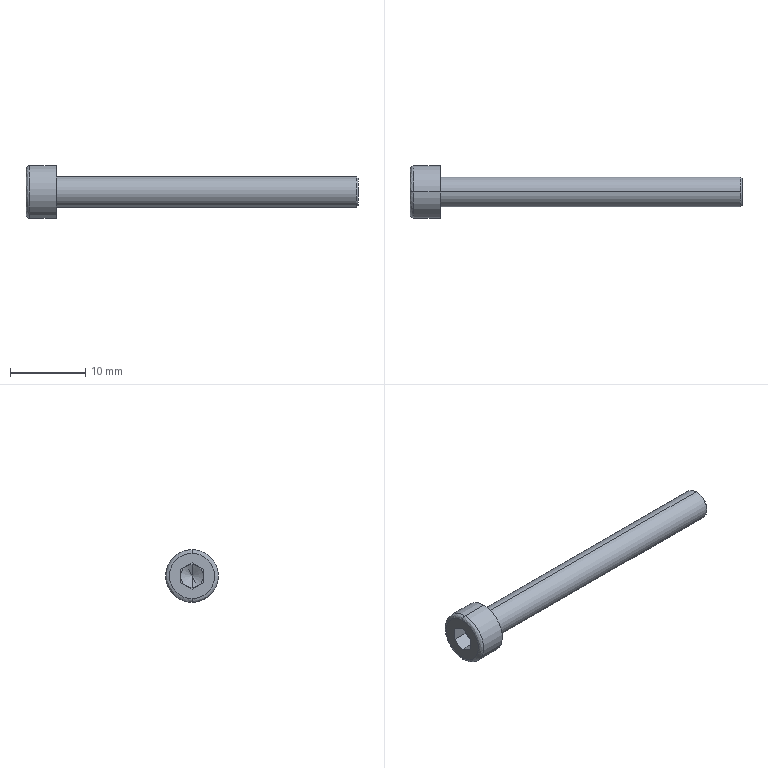Part | STEP file | hexagon socket head cap screws gb_GB_FASTENER_SCREWS_HSHCS M4X40-N | 1 solid | 25 faces | box 44 x 7 x 7 mm | volume 637.59 mm3 | plane 15 | cylinder 4 | cone 4 | spline 2 | commonest cylinder face diameters 4 x2 7 x2
STEP:
#1=CARTESIAN_POINT('',(0.5,0.,3.5));
#2=VERTEX_POINT('',#1);
#3=CARTESIAN_POINT('',(0.5,0.,-3.5));
#4=VERTEX_POINT('',#3);
#5=CARTESIAN_POINT('',(0.5,0.,0.));
#6=DIRECTION('',(1.,0.,0.));
#7=DIRECTION('',(0.,0.,1.));
#8=AXIS2_PLACEMENT_3D('',#5,#6,#7);
#9=CIRCLE('',#8,3.5);
#10=EDGE_CURVE('',#2,#4,#9,.T.);
#11=ORIENTED_EDGE('',*,*,#10,.F.);
#12=CARTESIAN_POINT('',(0.,0.,3.));
#13=VERTEX_POINT('',#12);
#14=CARTESIAN_POINT('',(0.5,0.,3.));
#15=DIRECTION('',(0.,-1.,0.));
#16=DIRECTION('',(0.,0.,1.));
#17=AXIS2_PLACEMENT_3D('',#14,#15,#16);
#18=CIRCLE('',#17,0.5);
#19=EDGE_CURVE('',#2,#13,#18,.T.);
#20=ORIENTED_EDGE('',*,*,#19,.T.);
#21=CARTESIAN_POINT('',(0.,0.,-3.));
#22=VERTEX_POINT('',#21);
#23=CARTESIAN_POINT('',(0.,0.,3.));
#24=CARTESIAN_POINT('',(0.,-6.,3.));
#25=CARTESIAN_POINT('',(0.,-6.,-3.));
#26=CARTESIAN_POINT('',(0.,0.,-3.));
#27=(BOUNDED_CURVE()B_SPLINE_CURVE(3,(#23,#24,#25,#26),.UNSPECIFIED.,.F.,.F.)B_SPLINE_CURVE_WITH_KNOTS((4,4),(0.,1.),.UNSPECIFIED.)CURVE()GEOMETRIC_REPRESENTATION_ITEM()RATIONAL_B_SPLINE_CURVE((1.,0.3333,0.3333,1.))REPRESENTATION_ITEM(''));
#28=EDGE_CURVE('',#13,#22,#27,.T.);
#29=ORIENTED_EDGE('',*,*,#28,.T.);
#30=CARTESIAN_POINT('',(0.5,0.,-3.));
#31=DIRECTION('',(0.,1.,0.));
#32=DIRECTION('',(0.,0.,-1.));
#33=AXIS2_PLACEMENT_3D('',#30,#31,#32);
#34=CIRCLE('',#33,0.5);
#35=EDGE_CURVE('',#4,#22,#34,.T.);
#36=ORIENTED_EDGE('',*,*,#35,.F.);
#37=EDGE_LOOP('',(#11,#20,#29,#36));
#38=FACE_OUTER_BOUND('',#37,.T.);
#39=CARTESIAN_POINT('',(0.5,0.,3.5));
#40=CARTESIAN_POINT('',(0.5,-7.,3.5));
#41=CARTESIAN_POINT('',(0.5,-7.,-3.5));
#42=CARTESIAN_POINT('',(0.5,0.,-3.5));
#43=CARTESIAN_POINT('',(0.2071,0.,3.5));
#44=CARTESIAN_POINT('',(0.2071,-7.,3.5));
#45=CARTESIAN_POINT('',(0.2071,-7.,-3.5));
#46=CARTESIAN_POINT('',(0.2071,0.,-3.5));
#47=CARTESIAN_POINT('',(0.,0.,3.293));
#48=CARTESIAN_POINT('',(0.,-6.586,3.293));
#49=CARTESIAN_POINT('',(0.,-6.586,-3.293));
#50=CARTESIAN_POINT('',(0.,0.,-3.293));
#51=CARTESIAN_POINT('',(0.,0.,3.));
#52=CARTESIAN_POINT('',(0.,-6.,3.));
#53=CARTESIAN_POINT('',(0.,-6.,-3.));
#54=CARTESIAN_POINT('',(0.,0.,-3.));
#55=(BOUNDED_SURFACE()B_SPLINE_SURFACE(3,3,((#39,#40,#41,#42),(#43,#44,#45,#46),(#47,#48,#49,#50),(#51,#52,#53,#54)),.UNSPECIFIED.,.F.,.F.,.F.)B_SPLINE_SURFACE_WITH_KNOTS((4,4),(4,4),(0.,1.),(0.,1.),.UNSPECIFIED.)GEOMETRIC_REPRESENTATION_ITEM()RATIONAL_B_SPLINE_SURFACE(((1.,0.3333,0.3333,1.),(0.8047,0.2682,0.2682,0.8047),(0.8047,0.2682,0.2682,0.8047),(1.,0.3333,0.3333,1.)))REPRESENTATION_ITEM('')SURFACE());
#56=ADVANCED_FACE('',(#38),#55,.T.);
#57=CARTESIAN_POINT('',(43.8,0.,2.));
#58=VERTEX_POINT('',#57);
#59=CARTESIAN_POINT('',(43.8,0.,-2.));
#60=VERTEX_POINT('',#59);
#61=CARTESIAN_POINT('',(43.8,0.,0.));
#62=DIRECTION('',(-1.,0.,0.));
#63=DIRECTION('',(0.,0.,1.));
#64=AXIS2_PLACEMENT_3D('',#61,#62,#63);
#65=CIRCLE('',#64,2.);
#66=EDGE_CURVE('',#58,#60,#65,.T.);
#67=ORIENTED_EDGE('',*,*,#66,.T.);
#68=CARTESIAN_POINT('',(4.,0.,-2.));
#69=VERTEX_POINT('',#68);
#70=CARTESIAN_POINT('',(44.,0.,-2.));
#71=DIRECTION('',(-1.,0.,0.));
#72=VECTOR('',#71,1000.);
#73=LINE('',#70,#72);
#74=EDGE_CURVE('',#60,#69,#73,.T.);
#75=ORIENTED_EDGE('',*,*,#74,.T.);
#76=CARTESIAN_POINT('',(4.,0.,2.));
#77=VERTEX_POINT('',#76);
#78=CARTESIAN_POINT('',(4.,0.,0.));
#79=DIRECTION('',(1.,0.,0.));
#80=DIRECTION('',(0.,0.,1.));
#81=AXIS2_PLACEMENT_3D('',#78,#79,#80);
#82=CIRCLE('',#81,2.);
#83=EDGE_CURVE('',#69,#77,#82,.T.);
#84=ORIENTED_EDGE('',*,*,#83,.T.);
#85=CARTESIAN_POINT('',(44.,0.,2.));
#86=DIRECTION('',(-1.,0.,0.));
#87=VECTOR('',#86,1000.);
#88=LINE('',#85,#87);
#89=EDGE_CURVE('',#58,#77,#88,.T.);
#90=ORIENTED_EDGE('',*,*,#89,.F.);
#91=EDGE_LOOP('',(#67,#75,#84,#90));
#92=FACE_OUTER_BOUND('',#91,.T.);
#93=CARTESIAN_POINT('',(44.,0.,0.));
#94=DIRECTION('',(-1.,0.,0.));
#95=DIRECTION('',(0.,0.,1.));
#96=AXIS2_PLACEMENT_3D('',#93,#94,#95);
#97=CYLINDRICAL_SURFACE('',#96,2.);
#98=ADVANCED_FACE('',(#92),#97,.T.);
#99=CARTESIAN_POINT('',(44.,0.,1.8));
#100=VERTEX_POINT('',#99);
#101=CARTESIAN_POINT('',(44.,0.,-1.8));
#102=VERTEX_POINT('',#101);
#103=CARTESIAN_POINT('',(44.,0.,0.));
#104=DIRECTION('',(-1.,0.,0.));
#105=DIRECTION('',(0.,0.,1.));
#106=AXIS2_PLACEMENT_3D('',#103,#104,#105);
#107=CIRCLE('',#106,1.8);
#108=EDGE_CURVE('',#100,#102,#107,.T.);
#109=ORIENTED_EDGE('',*,*,#108,.T.);
#110=CARTESIAN_POINT('',(43.8,0.,-2.));
#111=DIRECTION('',(-0.7071,0.,-0.7071));
#112=VECTOR('',#111,1000.);
#113=LINE('',#110,#112);
#114=EDGE_CURVE('',#102,#60,#113,.T.);
#115=ORIENTED_EDGE('',*,*,#114,.T.);
#116=ORIENTED_EDGE('',*,*,#66,.F.);
#117=CARTESIAN_POINT('',(43.8,0.,2.));
#118=DIRECTION('',(-0.7071,0.,0.7071));
#119=VECTOR('',#118,1000.);
#120=LINE('',#117,#119);
#121=EDGE_CURVE('',#100,#58,#120,.T.);
#122=ORIENTED_EDGE('',*,*,#121,.F.);
#123=EDGE_LOOP('',(#109,#115,#116,#122));
#124=FACE_OUTER_BOUND('',#123,.T.);
#125=CARTESIAN_POINT('',(43.8,0.,0.));
#126=DIRECTION('',(-1.,0.,0.));
#127=DIRECTION('',(0.,0.,1.));
#128=AXIS2_PLACEMENT_3D('',#125,#126,#127);
#129=CONICAL_SURFACE('',#128,2.,0.7854);
#130=ADVANCED_FACE('',(#124),#129,.T.);
#131=CARTESIAN_POINT('',(4.,0.,-3.5));
#132=VERTEX_POINT('',#131);
#133=CARTESIAN_POINT('',(4.,0.,3.5));
#134=VERTEX_POINT('',#133);
#135=CARTESIAN_POINT('',(4.,0.,0.));
#136=DIRECTION('',(1.,0.,0.));
#137=DIRECTION('',(0.,0.,1.));
#138=AXIS2_PLACEMENT_3D('',#135,#136,#137);
#139=CIRCLE('',#138,3.5);
#140=EDGE_CURVE('',#132,#134,#139,.T.);
#141=ORIENTED_EDGE('',*,*,#140,.F.);
#142=CARTESIAN_POINT('',(4.,0.,-3.5));
#143=DIRECTION('',(-1.,0.,0.));
#144=VECTOR('',#143,1000.);
#145=LINE('',#142,#144);
#146=EDGE_CURVE('',#132,#4,#145,.T.);
#147=ORIENTED_EDGE('',*,*,#146,.T.);
#148=CARTESIAN_POINT('',(0.5,0.,0.));
#149=DIRECTION('',(1.,0.,0.));
#150=DIRECTION('',(0.,0.,1.));
#151=AXIS2_PLACEMENT_3D('',#148,#149,#150);
#152=CIRCLE('',#151,3.5);
#153=EDGE_CURVE('',#4,#2,#152,.T.);
#154=ORIENTED_EDGE('',*,*,#153,.T.);
#155=CARTESIAN_POINT('',(4.,0.,3.5));
#156=DIRECTION('',(-1.,0.,0.));
#157=VECTOR('',#156,1000.);
#158=LINE('',#155,#157);
#159=EDGE_CURVE('',#134,#2,#158,.T.);
#160=ORIENTED_EDGE('',*,*,#159,.F.);
#161=EDGE_LOOP('',(#141,#147,#154,#160));
#162=FACE_OUTER_BOUND('',#161,.T.);
#163=CARTESIAN_POINT('',(4.,0.,0.));
#164=DIRECTION('',(-1.,0.,0.));
#165=DIRECTION('',(0.,0.,1.));
#166=AXIS2_PLACEMENT_3D('',#163,#164,#165);
#167=CYLINDRICAL_SURFACE('',#166,3.5);
#168=ADVANCED_FACE('',(#162),#167,.T.);
#169=CARTESIAN_POINT('',(2.866,0.,0.));
#170=VERTEX_POINT('',#169);
#171=CARTESIAN_POINT('',(2.,0.,1.5));
#172=VERTEX_POINT('',#171);
#173=CARTESIAN_POINT('',(2.,0.,1.5));
#174=DIRECTION('',(-0.5,0.,0.866));
#175=VECTOR('',#174,1000.);
#176=LINE('',#173,#175);
#177=EDGE_CURVE('',#170,#172,#176,.T.);
#178=ORIENTED_EDGE('',*,*,#177,.F.);
#179=CARTESIAN_POINT('',(2.,0.,-1.5));
#180=VERTEX_POINT('',#179);
#181=CARTESIAN_POINT('',(2.,0.,-1.5));
#182=DIRECTION('',(-0.5,0.,-0.866));
#183=VECTOR('',#182,1000.);
#184=LINE('',#181,#183);
#185=EDGE_CURVE('',#170,#180,#184,.T.);
#186=ORIENTED_EDGE('',*,*,#185,.T.);
#187=CARTESIAN_POINT('',(2.,-0.75,-1.299));
#188=VERTEX_POINT('',#187);
#189=CARTESIAN_POINT('',(2.,0.,0.));
#190=DIRECTION('',(1.,0.,0.));
#191=DIRECTION('',(0.,0.,1.));
#192=AXIS2_PLACEMENT_3D('',#189,#190,#191);
#193=CIRCLE('',#192,1.5);
#194=EDGE_CURVE('',#188,#180,#193,.T.);
#195=ORIENTED_EDGE('',*,*,#194,.F.);
#196=CARTESIAN_POINT('',(2.,-1.5,0.));
#197=VERTEX_POINT('',#196);
#198=CARTESIAN_POINT('',(2.,0.,0.));
#199=DIRECTION('',(1.,0.,0.));
#200=DIRECTION('',(0.,0.,1.));
#201=AXIS2_PLACEMENT_3D('',#198,#199,#200);
#202=CIRCLE('',#201,1.5);
#203=EDGE_CURVE('',#197,#188,#202,.T.);
#204=ORIENTED_EDGE('',*,*,#203,.F.);
#205=CARTESIAN_POINT('',(2.,-0.75,1.299));
#206=VERTEX_POINT('',#205);
#207=CARTESIAN_POINT('',(2.,0.,0.));
#208=DIRECTION('',(1.,0.,0.));
#209=DIRECTION('',(0.,0.,1.));
#210=AXIS2_PLACEMENT_3D('',#207,#208,#209);
#211=CIRCLE('',#210,1.5);
#212=EDGE_CURVE('',#206,#197,#211,.T.);
#213=ORIENTED_EDGE('',*,*,#212,.F.);
#214=CARTESIAN_POINT('',(2.,0.,0.));
#215=DIRECTION('',(1.,0.,0.));
#216=DIRECTION('',(0.,0.,1.));
#217=AXIS2_PLACEMENT_3D('',#214,#215,#216);
#218=CIRCLE('',#217,1.5);
#219=EDGE_CURVE('',#172,#206,#218,.T.);
#220=ORIENTED_EDGE('',*,*,#219,.F.);
#221=EDGE_LOOP('',(#178,#186,#195,#204,#213,#220));
#222=FACE_OUTER_BOUND('',#221,.T.);
#223=CARTESIAN_POINT('',(2.,0.,0.));
#224=DIRECTION('',(-1.,0.,0.));
#225=DIRECTION('',(0.,0.,1.));
#226=AXIS2_PLACEMENT_3D('',#223,#224,#225);
#227=CONICAL_SURFACE('',#226,1.5,1.047);
#228=ADVANCED_FACE('',(#222),#227,.F.);
#229=ORIENTED_EDGE('',*,*,#74,.F.);
#230=CARTESIAN_POINT('',(43.8,0.,0.));
#231=DIRECTION('',(-1.,0.,0.));
#232=DIRECTION('',(0.,0.,1.));
#233=AXIS2_PLACEMENT_3D('',#230,#231,#232);
#234=CIRCLE('',#233,2.);
#235=EDGE_CURVE('',#60,#58,#234,.T.);
#236=ORIENTED_EDGE('',*,*,#235,.T.);
#237=ORIENTED_EDGE('',*,*,#89,.T.);
#238=CARTESIAN_POINT('',(4.,0.,0.));
#239=DIRECTION('',(1.,0.,0.));
#240=DIRECTION('',(0.,0.,1.));
#241=AXIS2_PLACEMENT_3D('',#238,#239,#240);
#242=CIRCLE('',#241,2.);
#243=EDGE_CURVE('',#77,#69,#242,.T.);
#244=ORIENTED_EDGE('',*,*,#243,.T.);
#245=EDGE_LOOP('',(#229,#236,#237,#244));
#246=FACE_OUTER_BOUND('',#245,.T.);
#247=CARTESIAN_POINT('',(44.,0.,0.));
#248=DIRECTION('',(-1.,0.,0.));
#249=DIRECTION('',(0.,0.,1.));
#250=AXIS2_PLACEMENT_3D('',#247,#248,#249);
#251=CYLINDRICAL_SURFACE('',#250,2.);
#252=ADVANCED_FACE('',(#246),#251,.T.);
#253=ORIENTED_EDGE('',*,*,#243,.F.);
#254=ORIENTED_EDGE('',*,*,#83,.F.);
#255=EDGE_LOOP('',(#253,#254));
#256=FACE_BOUND('',#255,.T.);
#257=CARTESIAN_POINT('',(4.,0.,0.));
#258=DIRECTION('',(1.,0.,0.));
#259=DIRECTION('',(0.,0.,1.));
#260=AXIS2_PLACEMENT_3D('',#257,#258,#259);
#261=CIRCLE('',#260,3.5);
#262=EDGE_CURVE('',#134,#132,#261,.T.);
#263=ORIENTED_EDGE('',*,*,#262,.T.);
#264=ORIENTED_EDGE('',*,*,#140,.T.);
#265=EDGE_LOOP('',(#263,#264));
#266=FACE_OUTER_BOUND('',#265,.T.);
#267=CARTESIAN_POINT('',(4.,0.,0.));
#268=DIRECTION('',(1.,0.,0.));
#269=DIRECTION('',(0.,0.,-1.));
#270=AXIS2_PLACEMENT_3D('',#267,#268,#269);
#271=PLANE('',#270);
#272=ADVANCED_FACE('',(#256,#266),#271,.T.);
#273=ORIENTED_EDGE('',*,*,#114,.F.);
#274=CARTESIAN_POINT('',(44.,0.,0.));
#275=DIRECTION('',(-1.,0.,0.));
#276=DIRECTION('',(0.,0.,1.));
#277=AXIS2_PLACEMENT_3D('',#274,#275,#276);
#278=CIRCLE('',#277,1.8);
#279=EDGE_CURVE('',#102,#100,#278,.T.);
#280=ORIENTED_EDGE('',*,*,#279,.T.);
#281=ORIENTED_EDGE('',*,*,#121,.T.);
#282=ORIENTED_EDGE('',*,*,#235,.F.);
#283=EDGE_LOOP('',(#273,#280,#281,#282));
#284=FACE_OUTER_BOUND('',#283,.T.);
#285=CARTESIAN_POINT('',(43.8,0.,0.));
#286=DIRECTION('',(-1.,0.,0.));
#287=DIRECTION('',(0.,0.,1.));
#288=AXIS2_PLACEMENT_3D('',#285,#286,#287);
#289=CONICAL_SURFACE('',#288,2.,0.7854);
#290=ADVANCED_FACE('',(#284),#289,.T.);
#291=ORIENTED_EDGE('',*,*,#146,.F.);
#292=ORIENTED_EDGE('',*,*,#262,.F.);
#293=ORIENTED_EDGE('',*,*,#159,.T.);
#294=ORIENTED_EDGE('',*,*,#10,.T.);
#295=EDGE_LOOP('',(#291,#292,#293,#294));
#296=FACE_OUTER_BOUND('',#295,.T.);
#297=CARTESIAN_POINT('',(4.,0.,0.));
#298=DIRECTION('',(-1.,0.,0.));
#299=DIRECTION('',(0.,0.,1.));
#300=AXIS2_PLACEMENT_3D('',#297,#298,#299);
#301=CYLINDRICAL_SURFACE('',#300,3.5);
#302=ADVANCED_FACE('',(#296),#301,.T.);
#303=ORIENTED_EDGE('',*,*,#108,.F.);
#304=ORIENTED_EDGE('',*,*,#279,.F.);
#305=EDGE_LOOP('',(#303,#304));
#306=FACE_OUTER_BOUND('',#305,.T.);
#307=CARTESIAN_POINT('',(44.,0.,0.));
#308=DIRECTION('',(1.,0.,0.));
#309=DIRECTION('',(0.,0.,-1.));
#310=AXIS2_PLACEMENT_3D('',#307,#308,#309);
#311=PLANE('',#310);
#312=ADVANCED_FACE('',(#306),#311,.T.);
#313=ORIENTED_EDGE('',*,*,#19,.F.);
#314=ORIENTED_EDGE('',*,*,#153,.F.);
#315=ORIENTED_EDGE('',*,*,#35,.T.);
#316=CARTESIAN_POINT('',(0.,0.,-3.));
#317=CARTESIAN_POINT('',(0.,6.,-3.));
#318=CARTESIAN_POINT('',(0.,6.,3.));
#319=CARTESIAN_POINT('',(0.,0.,3.));
#320=(BOUNDED_CURVE()B_SPLINE_CURVE(3,(#316,#317,#318,#319),.UNSPECIFIED.,.F.,.F.)B_SPLINE_CURVE_WITH_KNOTS((4,4),(0.,1.),.UNSPECIFIED.)CURVE()GEOMETRIC_REPRESENTATION_ITEM()RATIONAL_B_SPLINE_CURVE((1.,0.3333,0.3333,1.))REPRESENTATION_ITEM(''));
#321=EDGE_CURVE('',#22,#13,#320,.T.);
#322=ORIENTED_EDGE('',*,*,#321,.T.);
#323=EDGE_LOOP('',(#313,#314,#315,#322));
#324=FACE_OUTER_BOUND('',#323,.T.);
#325=CARTESIAN_POINT('',(0.5,0.,-3.5));
#326=CARTESIAN_POINT('',(0.5,7.,-3.5));
#327=CARTESIAN_POINT('',(0.5,7.,3.5));
#328=CARTESIAN_POINT('',(0.5,0.,3.5));
#329=CARTESIAN_POINT('',(0.2071,0.,-3.5));
#330=CARTESIAN_POINT('',(0.2071,7.,-3.5));
#331=CARTESIAN_POINT('',(0.2071,7.,3.5));
#332=CARTESIAN_POINT('',(0.2071,0.,3.5));
#333=CARTESIAN_POINT('',(0.,0.,-3.293));
#334=CARTESIAN_POINT('',(0.,6.586,-3.293));
#335=CARTESIAN_POINT('',(0.,6.586,3.293));
#336=CARTESIAN_POINT('',(0.,0.,3.293));
#337=CARTESIAN_POINT('',(0.,0.,-3.));
#338=CARTESIAN_POINT('',(0.,6.,-3.));
#339=CARTESIAN_POINT('',(0.,6.,3.));
#340=CARTESIAN_POINT('',(0.,0.,3.));
#341=(BOUNDED_SURFACE()B_SPLINE_SURFACE(3,3,((#325,#326,#327,#328),(#329,#330,#331,#332),(#333,#334,#335,#336),(#337,#338,#339,#340)),.UNSPECIFIED.,.F.,.F.,.F.)B_SPLINE_SURFACE_WITH_KNOTS((4,4),(4,4),(0.,1.),(0.,1.),.UNSPECIFIED.)GEOMETRIC_REPRESENTATION_ITEM()RATIONAL_B_SPLINE_SURFACE(((1.,0.3333,0.3333,1.),(0.8047,0.2682,0.2682,0.8047),(0.8047,0.2682,0.2682,0.8047),(1.,0.3333,0.3333,1.)))REPRESENTATION_ITEM('')SURFACE());
#342=ADVANCED_FACE('',(#324),#341,.T.);
#343=CARTESIAN_POINT('',(0.,1.5,-0.866));
#344=VERTEX_POINT('',#343);
#345=CARTESIAN_POINT('',(0.,0.,-1.732));
#346=VERTEX_POINT('',#345);
#347=CARTESIAN_POINT('',(0.,0.,-1.732));
#348=DIRECTION('',(0.,-0.866,-0.5));
#349=VECTOR('',#348,1000.);
#350=LINE('',#347,#349);
#351=EDGE_CURVE('',#344,#346,#350,.T.);
#352=ORIENTED_EDGE('',*,*,#351,.F.);
#353=CARTESIAN_POINT('',(0.,1.5,0.866));
#354=VERTEX_POINT('',#353);
#355=CARTESIAN_POINT('',(0.,1.5,-0.866));
#356=DIRECTION('',(0.,0.,-1.));
#357=VECTOR('',#356,1000.);
#358=LINE('',#355,#357);
#359=EDGE_CURVE('',#354,#344,#358,.T.);
#360=ORIENTED_EDGE('',*,*,#359,.F.);
#361=CARTESIAN_POINT('',(0.,0.,1.732));
#362=VERTEX_POINT('',#361);
#363=CARTESIAN_POINT('',(0.,1.5,0.866));
#364=DIRECTION('',(0.,0.866,-0.5));
#365=VECTOR('',#364,1000.);
#366=LINE('',#363,#365);
#367=EDGE_CURVE('',#362,#354,#366,.T.);
#368=ORIENTED_EDGE('',*,*,#367,.F.);
#369=CARTESIAN_POINT('',(0.,-1.5,0.866));
#370=VERTEX_POINT('',#369);
#371=CARTESIAN_POINT('',(0.,0.,1.732));
#372=DIRECTION('',(0.,0.866,0.5));
#373=VECTOR('',#372,1000.);
#374=LINE('',#371,#373);
#375=EDGE_CURVE('',#370,#362,#374,.T.);
#376=ORIENTED_EDGE('',*,*,#375,.F.);
#377=CARTESIAN_POINT('',(0.,-1.5,-0.866));
#378=VERTEX_POINT('',#377);
#379=CARTESIAN_POINT('',(0.,-1.5,0.866));
#380=DIRECTION('',(0.,0.,1.));
#381=VECTOR('',#380,1000.);
#382=LINE('',#379,#381);
#383=EDGE_CURVE('',#378,#370,#382,.T.);
#384=ORIENTED_EDGE('',*,*,#383,.F.);
#385=CARTESIAN_POINT('',(0.,0.,-1.732));
#386=DIRECTION('',(0.,-0.866,0.5));
#387=VECTOR('',#386,1000.);
#388=LINE('',#385,#387);
#389=EDGE_CURVE('',#346,#378,#388,.T.);
#390=ORIENTED_EDGE('',*,*,#389,.F.);
#391=EDGE_LOOP('',(#352,#360,#368,#376,#384,#390));
#392=FACE_BOUND('',#391,.T.);
#393=ORIENTED_EDGE('',*,*,#321,.F.);
#394=ORIENTED_EDGE('',*,*,#28,.F.);
#395=EDGE_LOOP('',(#393,#394));
#396=FACE_OUTER_BOUND('',#395,.T.);
#397=CARTESIAN_POINT('',(0.,0.,0.));
#398=DIRECTION('',(1.,0.,0.));
#399=DIRECTION('',(0.,0.,-1.));
#400=AXIS2_PLACEMENT_3D('',#397,#398,#399);
#401=PLANE('',#400);
#402=ADVANCED_FACE('',(#392,#396),#401,.F.);
#403=CARTESIAN_POINT('',(2.,0.,-1.732));
#404=VERTEX_POINT('',#403);
#405=CARTESIAN_POINT('',(2.,-1.5,-0.866));
#406=DIRECTION('',(0.,0.866,-0.5));
#407=VECTOR('',#406,1000.);
#408=LINE('',#405,#407);
#409=EDGE_CURVE('',#188,#404,#408,.T.);
#410=ORIENTED_EDGE('',*,*,#409,.T.);
#411=CARTESIAN_POINT('',(2.,0.,-1.732));
#412=DIRECTION('',(-1.,0.,0.));
#413=VECTOR('',#412,1000.);
#414=LINE('',#411,#413);
#415=EDGE_CURVE('',#404,#346,#414,.T.);
#416=ORIENTED_EDGE('',*,*,#415,.T.);
#417=ORIENTED_EDGE('',*,*,#389,.T.);
#418=CARTESIAN_POINT('',(2.,-1.5,-0.866));
#419=VERTEX_POINT('',#418);
#420=CARTESIAN_POINT('',(2.,-1.5,-0.866));
#421=DIRECTION('',(1.,0.,0.));
#422=VECTOR('',#421,1000.);
#423=LINE('',#420,#422);
#424=EDGE_CURVE('',#378,#419,#423,.T.);
#425=ORIENTED_EDGE('',*,*,#424,.T.);
#426=CARTESIAN_POINT('',(2.,-1.5,-0.866));
#427=DIRECTION('',(0.,0.866,-0.5));
#428=VECTOR('',#427,1000.);
#429=LINE('',#426,#428);
#430=EDGE_CURVE('',#419,#188,#429,.T.);
#431=ORIENTED_EDGE('',*,*,#430,.T.);
#432=EDGE_LOOP('',(#410,#416,#417,#425,#431));
#433=FACE_OUTER_BOUND('',#432,.T.);
#434=CARTESIAN_POINT('',(2.,-1.5,-0.866));
#435=DIRECTION('',(0.,0.5,0.866));
#436=DIRECTION('',(0.,-0.866,0.5));
#437=AXIS2_PLACEMENT_3D('',#434,#435,#436);
#438=PLANE('',#437);
#439=ADVANCED_FACE('',(#433),#438,.T.);
#440=CARTESIAN_POINT('',(2.,0.75,-1.299));
#441=VERTEX_POINT('',#440);
#442=CARTESIAN_POINT('',(2.,1.5,-0.866));
#443=VERTEX_POINT('',#442);
#444=CARTESIAN_POINT('',(2.,0.,-1.732));
#445=DIRECTION('',(0.,0.866,0.5));
#446=VECTOR('',#445,1000.);
#447=LINE('',#444,#446);
#448=EDGE_CURVE('',#441,#443,#447,.T.);
#449=ORIENTED_EDGE('',*,*,#448,.T.);
#450=CARTESIAN_POINT('',(2.,1.5,-0.866));
#451=DIRECTION('',(-1.,0.,0.));
#452=VECTOR('',#451,1000.);
#453=LINE('',#450,#452);
#454=EDGE_CURVE('',#443,#344,#453,.T.);
#455=ORIENTED_EDGE('',*,*,#454,.T.);
#456=ORIENTED_EDGE('',*,*,#351,.T.);
#457=ORIENTED_EDGE('',*,*,#415,.F.);
#458=CARTESIAN_POINT('',(2.,0.,-1.732));
#459=DIRECTION('',(0.,0.866,0.5));
#460=VECTOR('',#459,1000.);
#461=LINE('',#458,#460);
#462=EDGE_CURVE('',#404,#441,#461,.T.);
#463=ORIENTED_EDGE('',*,*,#462,.T.);
#464=EDGE_LOOP('',(#449,#455,#456,#457,#463));
#465=FACE_OUTER_BOUND('',#464,.T.);
#466=CARTESIAN_POINT('',(2.,0.,-1.732));
#467=DIRECTION('',(0.,-0.5,0.866));
#468=DIRECTION('',(0.,-0.866,-0.5));
#469=AXIS2_PLACEMENT_3D('',#466,#467,#468);
#470=PLANE('',#469);
#471=ADVANCED_FACE('',(#465),#470,.T.);
#472=ORIENTED_EDGE('',*,*,#194,.T.);
#473=CARTESIAN_POINT('',(2.,0.,0.));
#474=DIRECTION('',(1.,0.,0.));
#475=DIRECTION('',(0.,0.,1.));
#476=AXIS2_PLACEMENT_3D('',#473,#474,#475);
#477=CIRCLE('',#476,1.5);
#478=EDGE_CURVE('',#180,#441,#477,.T.);
#479=ORIENTED_EDGE('',*,*,#478,.T.);
#480=ORIENTED_EDGE('',*,*,#462,.F.);
#481=ORIENTED_EDGE('',*,*,#409,.F.);
#482=EDGE_LOOP('',(#472,#479,#480,#481));
#483=FACE_OUTER_BOUND('',#482,.T.);
#484=CARTESIAN_POINT('',(2.,-3.,0.));
#485=DIRECTION('',(-1.,0.,0.));
#486=DIRECTION('',(0.,0.,1.));
#487=AXIS2_PLACEMENT_3D('',#484,#485,#486);
#488=PLANE('',#487);
#489=ADVANCED_FACE('',(#483),#488,.T.);
#490=ORIENTED_EDGE('',*,*,#203,.T.);
#491=ORIENTED_EDGE('',*,*,#430,.F.);
#492=CARTESIAN_POINT('',(2.,-1.5,0.));
#493=DIRECTION('',(0.,0.,1.));
#494=VECTOR('',#493,1000.);
#495=LINE('',#492,#494);
#496=EDGE_CURVE('',#419,#197,#495,.T.);
#497=ORIENTED_EDGE('',*,*,#496,.T.);
#498=EDGE_LOOP('',(#490,#491,#497));
#499=FACE_OUTER_BOUND('',#498,.T.);
#500=CARTESIAN_POINT('',(2.,-3.,0.));
#501=DIRECTION('',(-1.,0.,0.));
#502=DIRECTION('',(0.,0.,1.));
#503=AXIS2_PLACEMENT_3D('',#500,#501,#502);
#504=PLANE('',#503);
#505=ADVANCED_FACE('',(#499),#504,.T.);
#506=ORIENTED_EDGE('',*,*,#496,.F.);
#507=ORIENTED_EDGE('',*,*,#424,.F.);
#508=ORIENTED_EDGE('',*,*,#383,.T.);
#509=CARTESIAN_POINT('',(2.,-1.5,0.866));
#510=VERTEX_POINT('',#509);
#511=CARTESIAN_POINT('',(2.,-1.5,0.866));
#512=DIRECTION('',(1.,0.,0.));
#513=VECTOR('',#512,1000.);
#514=LINE('',#511,#513);
#515=EDGE_CURVE('',#370,#510,#514,.T.);
#516=ORIENTED_EDGE('',*,*,#515,.T.);
#517=CARTESIAN_POINT('',(2.,-1.5,0.866));
#518=DIRECTION('',(0.,0.,-1.));
#519=VECTOR('',#518,1000.);
#520=LINE('',#517,#519);
#521=EDGE_CURVE('',#510,#197,#520,.T.);
#522=ORIENTED_EDGE('',*,*,#521,.T.);
#523=EDGE_LOOP('',(#506,#507,#508,#516,#522));
#524=FACE_OUTER_BOUND('',#523,.T.);
#525=CARTESIAN_POINT('',(2.,-1.5,0.866));
#526=DIRECTION('',(0.,1.,0.));
#527=DIRECTION('',(0.,0.,1.));
#528=AXIS2_PLACEMENT_3D('',#525,#526,#527);
#529=PLANE('',#528);
#530=ADVANCED_FACE('',(#524),#529,.T.);
#531=CARTESIAN_POINT('',(2.,1.5,0.));
#532=VERTEX_POINT('',#531);
#533=CARTESIAN_POINT('',(2.,1.5,0.866));
#534=VERTEX_POINT('',#533);
#535=CARTESIAN_POINT('',(2.,1.5,-0.866));
#536=DIRECTION('',(0.,0.,1.));
#537=VECTOR('',#536,1000.);
#538=LINE('',#535,#537);
#539=EDGE_CURVE('',#532,#534,#538,.T.);
#540=ORIENTED_EDGE('',*,*,#539,.T.);
#541=CARTESIAN_POINT('',(2.,1.5,0.866));
#542=DIRECTION('',(-1.,0.,0.));
#543=VECTOR('',#542,1000.);
#544=LINE('',#541,#543);
#545=EDGE_CURVE('',#534,#354,#544,.T.);
#546=ORIENTED_EDGE('',*,*,#545,.T.);
#547=ORIENTED_EDGE('',*,*,#359,.T.);
#548=ORIENTED_EDGE('',*,*,#454,.F.);
#549=CARTESIAN_POINT('',(2.,1.5,-0.866));
#550=DIRECTION('',(0.,0.,1.));
#551=VECTOR('',#550,1000.);
#552=LINE('',#549,#551);
#553=EDGE_CURVE('',#443,#532,#552,.T.);
#554=ORIENTED_EDGE('',*,*,#553,.T.);
#555=EDGE_LOOP('',(#540,#546,#547,#548,#554));
#556=FACE_OUTER_BOUND('',#555,.T.);
#557=CARTESIAN_POINT('',(2.,1.5,-0.866));
#558=DIRECTION('',(0.,-1.,0.));
#559=DIRECTION('',(0.,0.,-1.));
#560=AXIS2_PLACEMENT_3D('',#557,#558,#559);
#561=PLANE('',#560);
#562=ADVANCED_FACE('',(#556),#561,.T.);
#563=CARTESIAN_POINT('',(2.,0.,0.));
#564=DIRECTION('',(1.,0.,0.));
#565=DIRECTION('',(0.,0.,1.));
#566=AXIS2_PLACEMENT_3D('',#563,#564,#565);
#567=CIRCLE('',#566,1.5);
#568=EDGE_CURVE('',#441,#532,#567,.T.);
#569=ORIENTED_EDGE('',*,*,#568,.T.);
#570=ORIENTED_EDGE('',*,*,#553,.F.);
#571=ORIENTED_EDGE('',*,*,#448,.F.);
#572=EDGE_LOOP('',(#569,#570,#571));
#573=FACE_OUTER_BOUND('',#572,.T.);
#574=CARTESIAN_POINT('',(2.,-3.,0.));
#575=DIRECTION('',(-1.,0.,0.));
#576=DIRECTION('',(0.,0.,1.));
#577=AXIS2_PLACEMENT_3D('',#574,#575,#576);
#578=PLANE('',#577);
#579=ADVANCED_FACE('',(#573),#578,.T.);
#580=ORIENTED_EDGE('',*,*,#185,.F.);
#581=ORIENTED_EDGE('',*,*,#177,.T.);
#582=CARTESIAN_POINT('',(2.,0.75,1.299));
#583=VERTEX_POINT('',#582);
#584=CARTESIAN_POINT('',(2.,0.,0.));
#585=DIRECTION('',(1.,0.,0.));
#586=DIRECTION('',(0.,0.,1.));
#587=AXIS2_PLACEMENT_3D('',#584,#585,#586);
#588=CIRCLE('',#587,1.5);
#589=EDGE_CURVE('',#583,#172,#588,.T.);
#590=ORIENTED_EDGE('',*,*,#589,.F.);
#591=CARTESIAN_POINT('',(2.,0.,0.));
#592=DIRECTION('',(1.,0.,0.));
#593=DIRECTION('',(0.,0.,1.));
#594=AXIS2_PLACEMENT_3D('',#591,#592,#593);
#595=CIRCLE('',#594,1.5);
#596=EDGE_CURVE('',#532,#583,#595,.T.);
#597=ORIENTED_EDGE('',*,*,#596,.F.);
#598=ORIENTED_EDGE('',*,*,#568,.F.);
#599=ORIENTED_EDGE('',*,*,#478,.F.);
#600=EDGE_LOOP('',(#580,#581,#590,#597,#598,#599));
#601=FACE_OUTER_BOUND('',#600,.T.);
#602=CARTESIAN_POINT('',(2.,0.,0.));
#603=DIRECTION('',(-1.,0.,0.));
#604=DIRECTION('',(0.,0.,1.));
#605=AXIS2_PLACEMENT_3D('',#602,#603,#604);
#606=CONICAL_SURFACE('',#605,1.5,1.047);
#607=ADVANCED_FACE('',(#601),#606,.F.);
#608=ORIENTED_EDGE('',*,*,#212,.T.);
#609=ORIENTED_EDGE('',*,*,#521,.F.);
#610=CARTESIAN_POINT('',(2.,-1.5,0.866));
#611=DIRECTION('',(0.,0.866,0.5));
#612=VECTOR('',#611,1000.);
#613=LINE('',#610,#612);
#614=EDGE_CURVE('',#510,#206,#613,.T.);
#615=ORIENTED_EDGE('',*,*,#614,.T.);
#616=EDGE_LOOP('',(#608,#609,#615));
#617=FACE_OUTER_BOUND('',#616,.T.);
#618=CARTESIAN_POINT('',(2.,-3.,0.));
#619=DIRECTION('',(-1.,0.,0.));
#620=DIRECTION('',(0.,0.,1.));
#621=AXIS2_PLACEMENT_3D('',#618,#619,#620);
#622=PLANE('',#621);
#623=ADVANCED_FACE('',(#617),#622,.T.);
#624=ORIENTED_EDGE('',*,*,#614,.F.);
#625=ORIENTED_EDGE('',*,*,#515,.F.);
#626=ORIENTED_EDGE('',*,*,#375,.T.);
#627=CARTESIAN_POINT('',(2.,0.,1.732));
#628=VERTEX_POINT('',#627);
#629=CARTESIAN_POINT('',(2.,0.,1.732));
#630=DIRECTION('',(1.,0.,0.));
#631=VECTOR('',#630,1000.);
#632=LINE('',#629,#631);
#633=EDGE_CURVE('',#362,#628,#632,.T.);
#634=ORIENTED_EDGE('',*,*,#633,.T.);
#635=CARTESIAN_POINT('',(2.,0.,1.732));
#636=DIRECTION('',(0.,-0.866,-0.5));
#637=VECTOR('',#636,1000.);
#638=LINE('',#635,#637);
#639=EDGE_CURVE('',#628,#206,#638,.T.);
#640=ORIENTED_EDGE('',*,*,#639,.T.);
#641=EDGE_LOOP('',(#624,#625,#626,#634,#640));
#642=FACE_OUTER_BOUND('',#641,.T.);
#643=CARTESIAN_POINT('',(2.,0.,1.732));
#644=DIRECTION('',(0.,0.5,-0.866));
#645=DIRECTION('',(0.,0.866,0.5));
#646=AXIS2_PLACEMENT_3D('',#643,#644,#645);
#647=PLANE('',#646);
#648=ADVANCED_FACE('',(#642),#647,.T.);
#649=CARTESIAN_POINT('',(2.,1.5,0.866));
#650=DIRECTION('',(0.,-0.866,0.5));
#651=VECTOR('',#650,1000.);
#652=LINE('',#649,#651);
#653=EDGE_CURVE('',#583,#628,#652,.T.);
#654=ORIENTED_EDGE('',*,*,#653,.T.);
#655=ORIENTED_EDGE('',*,*,#633,.F.);
#656=ORIENTED_EDGE('',*,*,#367,.T.);
#657=ORIENTED_EDGE('',*,*,#545,.F.);
#658=CARTESIAN_POINT('',(2.,1.5,0.866));
#659=DIRECTION('',(0.,-0.866,0.5));
#660=VECTOR('',#659,1000.);
#661=LINE('',#658,#660);
#662=EDGE_CURVE('',#534,#583,#661,.T.);
#663=ORIENTED_EDGE('',*,*,#662,.T.);
#664=EDGE_LOOP('',(#654,#655,#656,#657,#663));
#665=FACE_OUTER_BOUND('',#664,.T.);
#666=CARTESIAN_POINT('',(2.,1.5,0.866));
#667=DIRECTION('',(0.,-0.5,-0.866));
#668=DIRECTION('',(0.,0.866,-0.5));
#669=AXIS2_PLACEMENT_3D('',#666,#667,#668);
#670=PLANE('',#669);
#671=ADVANCED_FACE('',(#665),#670,.T.);
#672=ORIENTED_EDGE('',*,*,#596,.T.);
#673=ORIENTED_EDGE('',*,*,#662,.F.);
#674=ORIENTED_EDGE('',*,*,#539,.F.);
#675=EDGE_LOOP('',(#672,#673,#674));
#676=FACE_OUTER_BOUND('',#675,.T.);
#677=CARTESIAN_POINT('',(2.,-3.,0.));
#678=DIRECTION('',(-1.,0.,0.));
#679=DIRECTION('',(0.,0.,1.));
#680=AXIS2_PLACEMENT_3D('',#677,#678,#679);
#681=PLANE('',#680);
#682=ADVANCED_FACE('',(#676),#681,.T.);
#683=ORIENTED_EDGE('',*,*,#589,.T.);
#684=ORIENTED_EDGE('',*,*,#219,.T.);
#685=ORIENTED_EDGE('',*,*,#639,.F.);
#686=ORIENTED_EDGE('',*,*,#653,.F.);
#687=EDGE_LOOP('',(#683,#684,#685,#686));
#688=FACE_OUTER_BOUND('',#687,.T.);
#689=CARTESIAN_POINT('',(2.,-3.,0.));
#690=DIRECTION('',(-1.,0.,0.));
#691=DIRECTION('',(0.,0.,1.));
#692=AXIS2_PLACEMENT_3D('',#689,#690,#691);
#693=PLANE('',#692);
#694=ADVANCED_FACE('',(#688),#693,.T.);
#695=CLOSED_SHELL('',(#56,#98,#130,#168,#228,#252,#272,#290,#302,#312,#342,#402,#439,#471,#489,#505,#530,#562,#579,#607,#623,#648,#671,#682,#694));
#696=MANIFOLD_SOLID_BREP('',#695);
#697=CARTESIAN_POINT('',(0.,0.,0.));
#698=DIRECTION('',(0.,0.,1.));
#699=DIRECTION('',(1.,0.,0.));
#700=AXIS2_PLACEMENT_3D('',#697,#698,#699);
#701=(LENGTH_UNIT()NAMED_UNIT(*)SI_UNIT(.MILLI.,.METRE.));
#702=UNCERTAINTY_MEASURE_WITH_UNIT(LENGTH_MEASURE(0.00001),#701,'','');
#703=(NAMED_UNIT(*)PLANE_ANGLE_UNIT()SI_UNIT($,.RADIAN.));
#704=(NAMED_UNIT(*)SI_UNIT($,.STERADIAN.)SOLID_ANGLE_UNIT());
#705=(GEOMETRIC_REPRESENTATION_CONTEXT(3)GLOBAL_UNCERTAINTY_ASSIGNED_CONTEXT((#702))GLOBAL_UNIT_ASSIGNED_CONTEXT((#701,#703,#704))REPRESENTATION_CONTEXT('',''));
#706=ADVANCED_BREP_SHAPE_REPRESENTATION('',(#696,#700),#705);